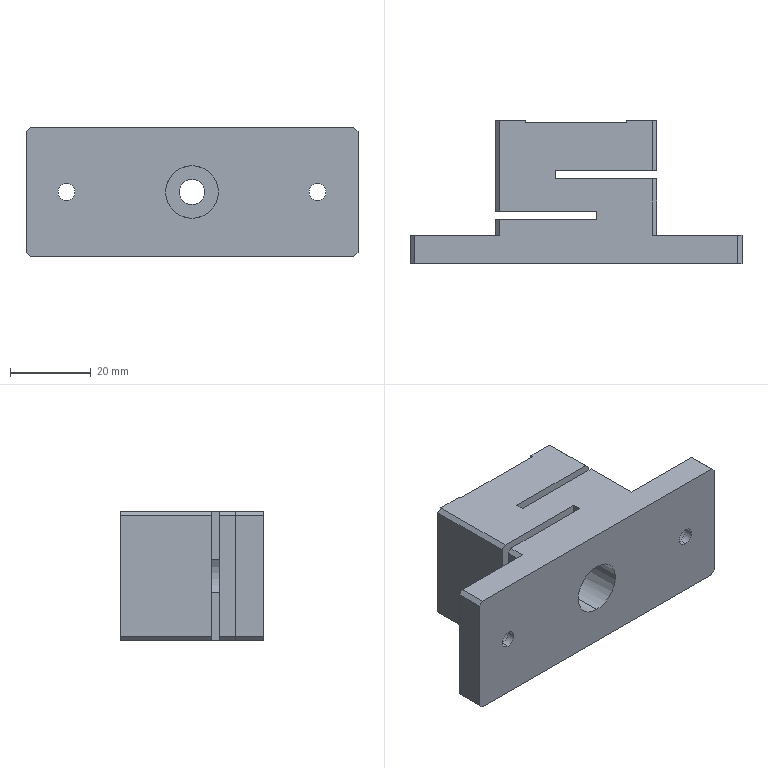Part | SolidWorks | features ICE 6, Chamfer 1, Extrusion 1 | 1 solid | 53 faces | box 82 x 35.5 x 32 mm | volume 46922 mm3 | plane 39 | cylinder 14 | commonest cylinder face diameters 4.2 x4 8.5 x4 13 x4 6.2 x2